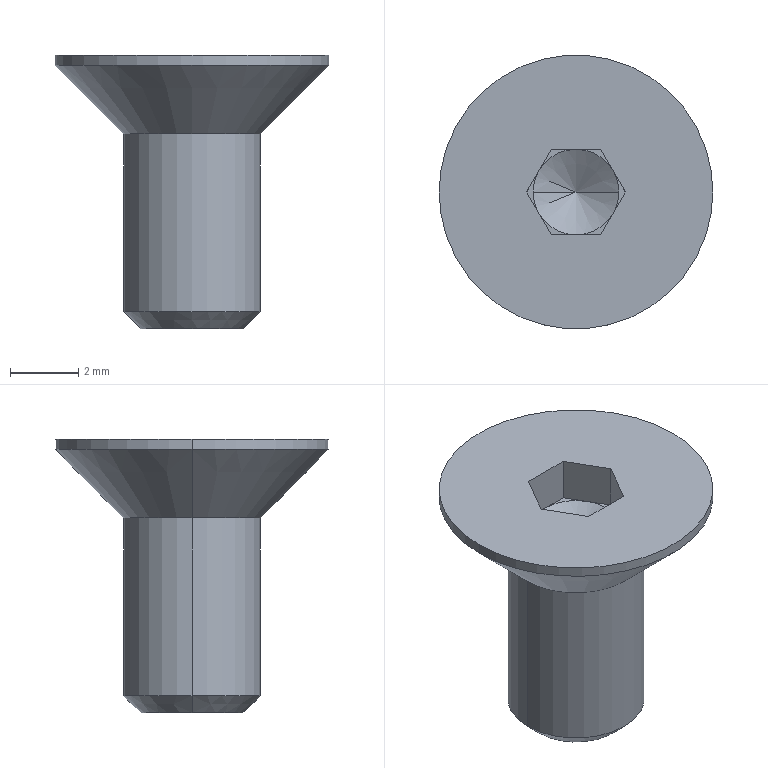Part | NX | features BREP 1 | 1 solid | 24 faces | box 8 x 8 x 8 mm | volume 135.694 mm3 | plane 14 | cone 6 | cylinder 4 | commonest cylinder face diameters 4 x2 8 x2
STEP:
#1=CARTESIAN_POINT('',(0.,0.,-2.022));
#2=VERTEX_POINT('',#1);
#3=CARTESIAN_POINT('',(-1.25,0.,-1.3));
#4=VERTEX_POINT('',#3);
#5=CARTESIAN_POINT('',(-1.25,0.,-1.3));
#6=DIRECTION('',(-0.866,0.,0.5));
#7=VECTOR('',#6,1000.);
#8=LINE('',#5,#7);
#9=EDGE_CURVE('',#2,#4,#8,.T.);
#10=ORIENTED_EDGE('',*,*,#9,.F.);
#11=CARTESIAN_POINT('',(1.25,0.,-1.3));
#12=VERTEX_POINT('',#11);
#13=CARTESIAN_POINT('',(1.25,0.,-1.3));
#14=DIRECTION('',(0.866,0.,0.5));
#15=VECTOR('',#14,1000.);
#16=LINE('',#13,#15);
#17=EDGE_CURVE('',#2,#12,#16,.T.);
#18=ORIENTED_EDGE('',*,*,#17,.T.);
#19=CARTESIAN_POINT('',(1.083,0.625,-1.3));
#20=VERTEX_POINT('',#19);
#21=CARTESIAN_POINT('',(0.,0.,-1.3));
#22=DIRECTION('',(0.,0.,-1.));
#23=DIRECTION('',(-1.,0.,0.));
#24=AXIS2_PLACEMENT_3D('',#21,#22,#23);
#25=CIRCLE('',#24,1.25);
#26=EDGE_CURVE('',#20,#12,#25,.T.);
#27=ORIENTED_EDGE('',*,*,#26,.F.);
#28=CARTESIAN_POINT('',(0.,1.25,-1.3));
#29=VERTEX_POINT('',#28);
#30=CARTESIAN_POINT('',(0.,0.,-1.3));
#31=DIRECTION('',(0.,0.,-1.));
#32=DIRECTION('',(-1.,0.,0.));
#33=AXIS2_PLACEMENT_3D('',#30,#31,#32);
#34=CIRCLE('',#33,1.25);
#35=EDGE_CURVE('',#29,#20,#34,.T.);
#36=ORIENTED_EDGE('',*,*,#35,.F.);
#37=CARTESIAN_POINT('',(-1.083,0.625,-1.3));
#38=VERTEX_POINT('',#37);
#39=CARTESIAN_POINT('',(0.,0.,-1.3));
#40=DIRECTION('',(0.,0.,-1.));
#41=DIRECTION('',(-1.,0.,0.));
#42=AXIS2_PLACEMENT_3D('',#39,#40,#41);
#43=CIRCLE('',#42,1.25);
#44=EDGE_CURVE('',#38,#29,#43,.T.);
#45=ORIENTED_EDGE('',*,*,#44,.F.);
#46=CARTESIAN_POINT('',(0.,0.,-1.3));
#47=DIRECTION('',(0.,0.,-1.));
#48=DIRECTION('',(-1.,0.,0.));
#49=AXIS2_PLACEMENT_3D('',#46,#47,#48);
#50=CIRCLE('',#49,1.25);
#51=EDGE_CURVE('',#4,#38,#50,.T.);
#52=ORIENTED_EDGE('',*,*,#51,.F.);
#53=EDGE_LOOP('',(#10,#18,#27,#36,#45,#52));
#54=FACE_BOUND('',#53,.T.);
#55=CARTESIAN_POINT('',(0.,0.,-1.3));
#56=DIRECTION('',(0.,0.,1.));
#57=DIRECTION('',(-1.,0.,0.));
#58=AXIS2_PLACEMENT_3D('',#55,#56,#57);
#59=CONICAL_SURFACE('',#58,1.25,1.047);
#60=ADVANCED_FACE('',(#54),#59,.F.);
#61=CARTESIAN_POINT('',(-1.5,0.,-8.));
#62=VERTEX_POINT('',#61);
#63=CARTESIAN_POINT('',(1.5,0.,-8.));
#64=VERTEX_POINT('',#63);
#65=CARTESIAN_POINT('',(0.,0.,-8.));
#66=DIRECTION('',(0.,0.,1.));
#67=DIRECTION('',(1.,0.,0.));
#68=AXIS2_PLACEMENT_3D('',#65,#66,#67);
#69=CIRCLE('',#68,1.5);
#70=EDGE_CURVE('',#62,#64,#69,.T.);
#71=ORIENTED_EDGE('',*,*,#70,.T.);
#72=CARTESIAN_POINT('',(2.,0.,-7.5));
#73=VERTEX_POINT('',#72);
#74=CARTESIAN_POINT('',(1.5,0.,-8.));
#75=DIRECTION('',(0.7071,0.,0.7071));
#76=VECTOR('',#75,1000.);
#77=LINE('',#74,#76);
#78=EDGE_CURVE('',#64,#73,#77,.T.);
#79=ORIENTED_EDGE('',*,*,#78,.T.);
#80=CARTESIAN_POINT('',(-2.,0.,-7.5));
#81=VERTEX_POINT('',#80);
#82=CARTESIAN_POINT('',(0.,0.,-7.5));
#83=DIRECTION('',(0.,0.,-1.));
#84=DIRECTION('',(1.,0.,0.));
#85=AXIS2_PLACEMENT_3D('',#82,#83,#84);
#86=CIRCLE('',#85,2.);
#87=EDGE_CURVE('',#73,#81,#86,.T.);
#88=ORIENTED_EDGE('',*,*,#87,.T.);
#89=CARTESIAN_POINT('',(-1.5,0.,-8.));
#90=DIRECTION('',(-0.7071,0.,0.7071));
#91=VECTOR('',#90,1000.);
#92=LINE('',#89,#91);
#93=EDGE_CURVE('',#62,#81,#92,.T.);
#94=ORIENTED_EDGE('',*,*,#93,.F.);
#95=EDGE_LOOP('',(#71,#79,#88,#94));
#96=FACE_BOUND('',#95,.T.);
#97=CARTESIAN_POINT('',(0.,0.,-8.));
#98=DIRECTION('',(0.,0.,1.));
#99=DIRECTION('',(-1.,0.,0.));
#100=AXIS2_PLACEMENT_3D('',#97,#98,#99);
#101=CONICAL_SURFACE('',#100,1.5,0.7854);
#102=ADVANCED_FACE('',(#96),#101,.T.);
#103=ORIENTED_EDGE('',*,*,#87,.F.);
#104=CARTESIAN_POINT('',(2.,0.,-2.3));
#105=VERTEX_POINT('',#104);
#106=CARTESIAN_POINT('',(2.,0.,-8.));
#107=DIRECTION('',(0.,0.,1.));
#108=VECTOR('',#107,1000.);
#109=LINE('',#106,#108);
#110=EDGE_CURVE('',#73,#105,#109,.T.);
#111=ORIENTED_EDGE('',*,*,#110,.T.);
#112=CARTESIAN_POINT('',(-2.,0.,-2.3));
#113=VERTEX_POINT('',#112);
#114=CARTESIAN_POINT('',(0.,0.,-2.3));
#115=DIRECTION('',(0.,0.,1.));
#116=DIRECTION('',(1.,0.,0.));
#117=AXIS2_PLACEMENT_3D('',#114,#115,#116);
#118=CIRCLE('',#117,2.);
#119=EDGE_CURVE('',#113,#105,#118,.T.);
#120=ORIENTED_EDGE('',*,*,#119,.F.);
#121=CARTESIAN_POINT('',(-2.,0.,-8.));
#122=DIRECTION('',(0.,0.,1.));
#123=VECTOR('',#122,1000.);
#124=LINE('',#121,#123);
#125=EDGE_CURVE('',#81,#113,#124,.T.);
#126=ORIENTED_EDGE('',*,*,#125,.F.);
#127=EDGE_LOOP('',(#103,#111,#120,#126));
#128=FACE_BOUND('',#127,.T.);
#129=CARTESIAN_POINT('',(0.,0.,-8.));
#130=DIRECTION('',(0.,0.,1.));
#131=DIRECTION('',(-1.,0.,0.));
#132=AXIS2_PLACEMENT_3D('',#129,#130,#131);
#133=CYLINDRICAL_SURFACE('',#132,2.);
#134=ADVANCED_FACE('',(#128),#133,.T.);
#135=ORIENTED_EDGE('',*,*,#119,.T.);
#136=CARTESIAN_POINT('',(4.,0.,-0.3));
#137=VERTEX_POINT('',#136);
#138=CARTESIAN_POINT('',(2.,0.,-2.3));
#139=DIRECTION('',(0.7071,0.,0.7071));
#140=VECTOR('',#139,1000.);
#141=LINE('',#138,#140);
#142=EDGE_CURVE('',#105,#137,#141,.T.);
#143=ORIENTED_EDGE('',*,*,#142,.T.);
#144=CARTESIAN_POINT('',(-4.,0.,-0.3));
#145=VERTEX_POINT('',#144);
#146=CARTESIAN_POINT('',(0.,0.,-0.3));
#147=DIRECTION('',(0.,0.,-1.));
#148=DIRECTION('',(1.,0.,0.));
#149=AXIS2_PLACEMENT_3D('',#146,#147,#148);
#150=CIRCLE('',#149,4.);
#151=EDGE_CURVE('',#137,#145,#150,.T.);
#152=ORIENTED_EDGE('',*,*,#151,.T.);
#153=CARTESIAN_POINT('',(-2.,0.,-2.3));
#154=DIRECTION('',(-0.7071,0.,0.7071));
#155=VECTOR('',#154,1000.);
#156=LINE('',#153,#155);
#157=EDGE_CURVE('',#113,#145,#156,.T.);
#158=ORIENTED_EDGE('',*,*,#157,.F.);
#159=EDGE_LOOP('',(#135,#143,#152,#158));
#160=FACE_BOUND('',#159,.T.);
#161=CARTESIAN_POINT('',(0.,0.,-2.3));
#162=DIRECTION('',(0.,0.,1.));
#163=DIRECTION('',(-1.,0.,0.));
#164=AXIS2_PLACEMENT_3D('',#161,#162,#163);
#165=CONICAL_SURFACE('',#164,2.,0.7854);
#166=ADVANCED_FACE('',(#160),#165,.T.);
#167=ORIENTED_EDGE('',*,*,#151,.F.);
#168=CARTESIAN_POINT('',(4.,0.,0.));
#169=VERTEX_POINT('',#168);
#170=CARTESIAN_POINT('',(4.,0.,-2.3));
#171=DIRECTION('',(0.,0.,1.));
#172=VECTOR('',#171,1000.);
#173=LINE('',#170,#172);
#174=EDGE_CURVE('',#137,#169,#173,.T.);
#175=ORIENTED_EDGE('',*,*,#174,.T.);
#176=CARTESIAN_POINT('',(-4.,0.,0.));
#177=VERTEX_POINT('',#176);
#178=CARTESIAN_POINT('',(0.,0.,0.));
#179=DIRECTION('',(0.,0.,1.));
#180=DIRECTION('',(1.,0.,0.));
#181=AXIS2_PLACEMENT_3D('',#178,#179,#180);
#182=CIRCLE('',#181,4.);
#183=EDGE_CURVE('',#177,#169,#182,.T.);
#184=ORIENTED_EDGE('',*,*,#183,.F.);
#185=CARTESIAN_POINT('',(-4.,0.,-2.3));
#186=DIRECTION('',(0.,0.,1.));
#187=VECTOR('',#186,1000.);
#188=LINE('',#185,#187);
#189=EDGE_CURVE('',#145,#177,#188,.T.);
#190=ORIENTED_EDGE('',*,*,#189,.F.);
#191=EDGE_LOOP('',(#167,#175,#184,#190));
#192=FACE_BOUND('',#191,.T.);
#193=CARTESIAN_POINT('',(0.,0.,-2.3));
#194=DIRECTION('',(0.,0.,1.));
#195=DIRECTION('',(-1.,0.,0.));
#196=AXIS2_PLACEMENT_3D('',#193,#194,#195);
#197=CYLINDRICAL_SURFACE('',#196,4.);
#198=ADVANCED_FACE('',(#192),#197,.T.);
#199=ORIENTED_EDGE('',*,*,#44,.T.);
#200=CARTESIAN_POINT('',(-0.7217,1.25,-1.3));
#201=VERTEX_POINT('',#200);
#202=CARTESIAN_POINT('',(-0.7217,1.25,-1.3));
#203=DIRECTION('',(1.,0.,0.));
#204=VECTOR('',#203,1000.);
#205=LINE('',#202,#204);
#206=EDGE_CURVE('',#201,#29,#205,.T.);
#207=ORIENTED_EDGE('',*,*,#206,.F.);
#208=CARTESIAN_POINT('',(-1.443,0.,-1.3));
#209=DIRECTION('',(0.5,0.866,0.));
#210=VECTOR('',#209,1000.);
#211=LINE('',#208,#210);
#212=EDGE_CURVE('',#38,#201,#211,.T.);
#213=ORIENTED_EDGE('',*,*,#212,.F.);
#214=EDGE_LOOP('',(#199,#207,#213));
#215=FACE_BOUND('',#214,.T.);
#216=CARTESIAN_POINT('',(0.,0.,-1.3));
#217=DIRECTION('',(0.,0.,1.));
#218=DIRECTION('',(1.,0.,0.));
#219=AXIS2_PLACEMENT_3D('',#216,#217,#218);
#220=PLANE('',#219);
#221=ADVANCED_FACE('',(#215),#220,.T.);
#222=ORIENTED_EDGE('',*,*,#35,.T.);
#223=CARTESIAN_POINT('',(0.7217,1.25,-1.3));
#224=VERTEX_POINT('',#223);
#225=CARTESIAN_POINT('',(0.7217,1.25,-1.3));
#226=DIRECTION('',(0.5,-0.866,0.));
#227=VECTOR('',#226,1000.);
#228=LINE('',#225,#227);
#229=EDGE_CURVE('',#224,#20,#228,.T.);
#230=ORIENTED_EDGE('',*,*,#229,.F.);
#231=CARTESIAN_POINT('',(-0.7217,1.25,-1.3));
#232=DIRECTION('',(1.,0.,0.));
#233=VECTOR('',#232,1000.);
#234=LINE('',#231,#233);
#235=EDGE_CURVE('',#29,#224,#234,.T.);
#236=ORIENTED_EDGE('',*,*,#235,.F.);
#237=EDGE_LOOP('',(#222,#230,#236));
#238=FACE_BOUND('',#237,.T.);
#239=CARTESIAN_POINT('',(0.,0.,-1.3));
#240=DIRECTION('',(0.,0.,1.));
#241=DIRECTION('',(1.,0.,0.));
#242=AXIS2_PLACEMENT_3D('',#239,#240,#241);
#243=PLANE('',#242);
#244=ADVANCED_FACE('',(#238),#243,.T.);
#245=ORIENTED_EDGE('',*,*,#26,.T.);
#246=CARTESIAN_POINT('',(1.083,-0.625,-1.3));
#247=VERTEX_POINT('',#246);
#248=CARTESIAN_POINT('',(0.,0.,-1.3));
#249=DIRECTION('',(0.,0.,-1.));
#250=DIRECTION('',(-1.,0.,0.));
#251=AXIS2_PLACEMENT_3D('',#248,#249,#250);
#252=CIRCLE('',#251,1.25);
#253=EDGE_CURVE('',#12,#247,#252,.T.);
#254=ORIENTED_EDGE('',*,*,#253,.T.);
#255=CARTESIAN_POINT('',(1.443,0.,-1.3));
#256=VERTEX_POINT('',#255);
#257=CARTESIAN_POINT('',(1.443,0.,-1.3));
#258=DIRECTION('',(-0.5,-0.866,0.));
#259=VECTOR('',#258,1000.);
#260=LINE('',#257,#259);
#261=EDGE_CURVE('',#256,#247,#260,.T.);
#262=ORIENTED_EDGE('',*,*,#261,.F.);
#263=CARTESIAN_POINT('',(0.7217,1.25,-1.3));
#264=DIRECTION('',(0.5,-0.866,0.));
#265=VECTOR('',#264,1000.);
#266=LINE('',#263,#265);
#267=EDGE_CURVE('',#20,#256,#266,.T.);
#268=ORIENTED_EDGE('',*,*,#267,.F.);
#269=EDGE_LOOP('',(#245,#254,#262,#268));
#270=FACE_BOUND('',#269,.T.);
#271=CARTESIAN_POINT('',(0.,0.,-1.3));
#272=DIRECTION('',(0.,0.,1.));
#273=DIRECTION('',(1.,0.,0.));
#274=AXIS2_PLACEMENT_3D('',#271,#272,#273);
#275=PLANE('',#274);
#276=ADVANCED_FACE('',(#270),#275,.T.);
#277=CARTESIAN_POINT('',(0.,-1.25,-1.3));
#278=VERTEX_POINT('',#277);
#279=CARTESIAN_POINT('',(0.,0.,-1.3));
#280=DIRECTION('',(0.,0.,-1.));
#281=DIRECTION('',(-1.,0.,0.));
#282=AXIS2_PLACEMENT_3D('',#279,#280,#281);
#283=CIRCLE('',#282,1.25);
#284=EDGE_CURVE('',#247,#278,#283,.T.);
#285=ORIENTED_EDGE('',*,*,#284,.T.);
#286=CARTESIAN_POINT('',(0.7217,-1.25,-1.3));
#287=VERTEX_POINT('',#286);
#288=CARTESIAN_POINT('',(0.7217,-1.25,-1.3));
#289=DIRECTION('',(-1.,0.,0.));
#290=VECTOR('',#289,1000.);
#291=LINE('',#288,#290);
#292=EDGE_CURVE('',#287,#278,#291,.T.);
#293=ORIENTED_EDGE('',*,*,#292,.F.);
#294=CARTESIAN_POINT('',(1.443,0.,-1.3));
#295=DIRECTION('',(-0.5,-0.866,0.));
#296=VECTOR('',#295,1000.);
#297=LINE('',#294,#296);
#298=EDGE_CURVE('',#247,#287,#297,.T.);
#299=ORIENTED_EDGE('',*,*,#298,.F.);
#300=EDGE_LOOP('',(#285,#293,#299));
#301=FACE_BOUND('',#300,.T.);
#302=CARTESIAN_POINT('',(0.,0.,-1.3));
#303=DIRECTION('',(0.,0.,1.));
#304=DIRECTION('',(1.,0.,0.));
#305=AXIS2_PLACEMENT_3D('',#302,#303,#304);
#306=PLANE('',#305);
#307=ADVANCED_FACE('',(#301),#306,.T.);
#308=CARTESIAN_POINT('',(-1.083,-0.625,-1.3));
#309=VERTEX_POINT('',#308);
#310=CARTESIAN_POINT('',(0.,0.,-1.3));
#311=DIRECTION('',(0.,0.,-1.));
#312=DIRECTION('',(-1.,0.,0.));
#313=AXIS2_PLACEMENT_3D('',#310,#311,#312);
#314=CIRCLE('',#313,1.25);
#315=EDGE_CURVE('',#278,#309,#314,.T.);
#316=ORIENTED_EDGE('',*,*,#315,.T.);
#317=CARTESIAN_POINT('',(-0.7217,-1.25,-1.3));
#318=VERTEX_POINT('',#317);
#319=CARTESIAN_POINT('',(-0.7217,-1.25,-1.3));
#320=DIRECTION('',(-0.5,0.866,0.));
#321=VECTOR('',#320,1000.);
#322=LINE('',#319,#321);
#323=EDGE_CURVE('',#318,#309,#322,.T.);
#324=ORIENTED_EDGE('',*,*,#323,.F.);
#325=CARTESIAN_POINT('',(0.7217,-1.25,-1.3));
#326=DIRECTION('',(-1.,0.,0.));
#327=VECTOR('',#326,1000.);
#328=LINE('',#325,#327);
#329=EDGE_CURVE('',#278,#318,#328,.T.);
#330=ORIENTED_EDGE('',*,*,#329,.F.);
#331=EDGE_LOOP('',(#316,#324,#330));
#332=FACE_BOUND('',#331,.T.);
#333=CARTESIAN_POINT('',(0.,0.,-1.3));
#334=DIRECTION('',(0.,0.,1.));
#335=DIRECTION('',(1.,0.,0.));
#336=AXIS2_PLACEMENT_3D('',#333,#334,#335);
#337=PLANE('',#336);
#338=ADVANCED_FACE('',(#332),#337,.T.);
#339=ORIENTED_EDGE('',*,*,#174,.F.);
#340=CARTESIAN_POINT('',(0.,0.,-0.3));
#341=DIRECTION('',(0.,0.,-1.));
#342=DIRECTION('',(1.,0.,0.));
#343=AXIS2_PLACEMENT_3D('',#340,#341,#342);
#344=CIRCLE('',#343,4.);
#345=EDGE_CURVE('',#145,#137,#344,.T.);
#346=ORIENTED_EDGE('',*,*,#345,.F.);
#347=ORIENTED_EDGE('',*,*,#189,.T.);
#348=CARTESIAN_POINT('',(0.,0.,0.));
#349=DIRECTION('',(0.,0.,1.));
#350=DIRECTION('',(1.,0.,0.));
#351=AXIS2_PLACEMENT_3D('',#348,#349,#350);
#352=CIRCLE('',#351,4.);
#353=EDGE_CURVE('',#169,#177,#352,.T.);
#354=ORIENTED_EDGE('',*,*,#353,.F.);
#355=EDGE_LOOP('',(#339,#346,#347,#354));
#356=FACE_BOUND('',#355,.T.);
#357=CARTESIAN_POINT('',(0.,0.,-2.3));
#358=DIRECTION('',(0.,0.,1.));
#359=DIRECTION('',(-1.,0.,0.));
#360=AXIS2_PLACEMENT_3D('',#357,#358,#359);
#361=CYLINDRICAL_SURFACE('',#360,4.);
#362=ADVANCED_FACE('',(#356),#361,.T.);
#363=ORIENTED_EDGE('',*,*,#183,.T.);
#364=ORIENTED_EDGE('',*,*,#353,.T.);
#365=EDGE_LOOP('',(#363,#364));
#366=FACE_BOUND('',#365,.T.);
#367=CARTESIAN_POINT('',(-0.7217,1.25,0.));
#368=VERTEX_POINT('',#367);
#369=CARTESIAN_POINT('',(0.7217,1.25,0.));
#370=VERTEX_POINT('',#369);
#371=CARTESIAN_POINT('',(-0.7217,1.25,0.));
#372=DIRECTION('',(1.,0.,0.));
#373=VECTOR('',#372,1000.);
#374=LINE('',#371,#373);
#375=EDGE_CURVE('',#368,#370,#374,.T.);
#376=ORIENTED_EDGE('',*,*,#375,.T.);
#377=CARTESIAN_POINT('',(1.443,0.,0.));
#378=VERTEX_POINT('',#377);
#379=CARTESIAN_POINT('',(0.7217,1.25,0.));
#380=DIRECTION('',(0.5,-0.866,0.));
#381=VECTOR('',#380,1000.);
#382=LINE('',#379,#381);
#383=EDGE_CURVE('',#370,#378,#382,.T.);
#384=ORIENTED_EDGE('',*,*,#383,.T.);
#385=CARTESIAN_POINT('',(0.7217,-1.25,0.));
#386=VERTEX_POINT('',#385);
#387=CARTESIAN_POINT('',(1.443,0.,0.));
#388=DIRECTION('',(-0.5,-0.866,0.));
#389=VECTOR('',#388,1000.);
#390=LINE('',#387,#389);
#391=EDGE_CURVE('',#378,#386,#390,.T.);
#392=ORIENTED_EDGE('',*,*,#391,.T.);
#393=CARTESIAN_POINT('',(-0.7217,-1.25,0.));
#394=VERTEX_POINT('',#393);
#395=CARTESIAN_POINT('',(0.7217,-1.25,0.));
#396=DIRECTION('',(-1.,0.,0.));
#397=VECTOR('',#396,1000.);
#398=LINE('',#395,#397);
#399=EDGE_CURVE('',#386,#394,#398,.T.);
#400=ORIENTED_EDGE('',*,*,#399,.T.);
#401=CARTESIAN_POINT('',(-1.443,0.,0.));
#402=VERTEX_POINT('',#401);
#403=CARTESIAN_POINT('',(-0.7217,-1.25,0.));
#404=DIRECTION('',(-0.5,0.866,0.));
#405=VECTOR('',#404,1000.);
#406=LINE('',#403,#405);
#407=EDGE_CURVE('',#394,#402,#406,.T.);
#408=ORIENTED_EDGE('',*,*,#407,.T.);
#409=CARTESIAN_POINT('',(-1.443,0.,0.));
#410=DIRECTION('',(0.5,0.866,0.));
#411=VECTOR('',#410,1000.);
#412=LINE('',#409,#411);
#413=EDGE_CURVE('',#402,#368,#412,.T.);
#414=ORIENTED_EDGE('',*,*,#413,.T.);
#415=EDGE_LOOP('',(#376,#384,#392,#400,#408,#414));
#416=FACE_BOUND('',#415,.T.);
#417=CARTESIAN_POINT('',(0.,0.,0.));
#418=DIRECTION('',(0.,0.,-1.));
#419=DIRECTION('',(0.,-1.,0.));
#420=AXIS2_PLACEMENT_3D('',#417,#418,#419);
#421=PLANE('',#420);
#422=ADVANCED_FACE('',(#366,#416),#421,.F.);
#423=ORIENTED_EDGE('',*,*,#142,.F.);
#424=CARTESIAN_POINT('',(0.,0.,-2.3));
#425=DIRECTION('',(0.,0.,1.));
#426=DIRECTION('',(1.,0.,0.));
#427=AXIS2_PLACEMENT_3D('',#424,#425,#426);
#428=CIRCLE('',#427,2.);
#429=EDGE_CURVE('',#105,#113,#428,.T.);
#430=ORIENTED_EDGE('',*,*,#429,.T.);
#431=ORIENTED_EDGE('',*,*,#157,.T.);
#432=ORIENTED_EDGE('',*,*,#345,.T.);
#433=EDGE_LOOP('',(#423,#430,#431,#432));
#434=FACE_BOUND('',#433,.T.);
#435=CARTESIAN_POINT('',(0.,0.,-2.3));
#436=DIRECTION('',(0.,0.,1.));
#437=DIRECTION('',(-1.,0.,0.));
#438=AXIS2_PLACEMENT_3D('',#435,#436,#437);
#439=CONICAL_SURFACE('',#438,2.,0.7854);
#440=ADVANCED_FACE('',(#434),#439,.T.);
#441=ORIENTED_EDGE('',*,*,#110,.F.);
#442=CARTESIAN_POINT('',(0.,0.,-7.5));
#443=DIRECTION('',(0.,0.,-1.));
#444=DIRECTION('',(1.,0.,0.));
#445=AXIS2_PLACEMENT_3D('',#442,#443,#444);
#446=CIRCLE('',#445,2.);
#447=EDGE_CURVE('',#81,#73,#446,.T.);
#448=ORIENTED_EDGE('',*,*,#447,.F.);
#449=ORIENTED_EDGE('',*,*,#125,.T.);
#450=ORIENTED_EDGE('',*,*,#429,.F.);
#451=EDGE_LOOP('',(#441,#448,#449,#450));
#452=FACE_BOUND('',#451,.T.);
#453=CARTESIAN_POINT('',(0.,0.,-8.));
#454=DIRECTION('',(0.,0.,1.));
#455=DIRECTION('',(-1.,0.,0.));
#456=AXIS2_PLACEMENT_3D('',#453,#454,#455);
#457=CYLINDRICAL_SURFACE('',#456,2.);
#458=ADVANCED_FACE('',(#452),#457,.T.);
#459=ORIENTED_EDGE('',*,*,#70,.F.);
#460=CARTESIAN_POINT('',(0.,0.,-8.));
#461=DIRECTION('',(0.,0.,1.));
#462=DIRECTION('',(1.,0.,0.));
#463=AXIS2_PLACEMENT_3D('',#460,#461,#462);
#464=CIRCLE('',#463,1.5);
#465=EDGE_CURVE('',#64,#62,#464,.T.);
#466=ORIENTED_EDGE('',*,*,#465,.F.);
#467=EDGE_LOOP('',(#459,#466));
#468=FACE_BOUND('',#467,.T.);
#469=CARTESIAN_POINT('',(0.,0.,-8.));
#470=DIRECTION('',(0.,0.,-1.));
#471=DIRECTION('',(0.,-1.,0.));
#472=AXIS2_PLACEMENT_3D('',#469,#470,#471);
#473=PLANE('',#472);
#474=ADVANCED_FACE('',(#468),#473,.T.);
#475=ORIENTED_EDGE('',*,*,#78,.F.);
#476=ORIENTED_EDGE('',*,*,#465,.T.);
#477=ORIENTED_EDGE('',*,*,#93,.T.);
#478=ORIENTED_EDGE('',*,*,#447,.T.);
#479=EDGE_LOOP('',(#475,#476,#477,#478));
#480=FACE_BOUND('',#479,.T.);
#481=CARTESIAN_POINT('',(0.,0.,-8.));
#482=DIRECTION('',(0.,0.,1.));
#483=DIRECTION('',(-1.,0.,0.));
#484=AXIS2_PLACEMENT_3D('',#481,#482,#483);
#485=CONICAL_SURFACE('',#484,1.5,0.7854);
#486=ADVANCED_FACE('',(#480),#485,.T.);
#487=ORIENTED_EDGE('',*,*,#413,.F.);
#488=CARTESIAN_POINT('',(-1.443,0.,-1.3));
#489=VERTEX_POINT('',#488);
#490=CARTESIAN_POINT('',(-1.443,0.,-1.3));
#491=DIRECTION('',(0.,0.,1.));
#492=VECTOR('',#491,1000.);
#493=LINE('',#490,#492);
#494=EDGE_CURVE('',#489,#402,#493,.T.);
#495=ORIENTED_EDGE('',*,*,#494,.F.);
#496=CARTESIAN_POINT('',(-1.443,0.,-1.3));
#497=DIRECTION('',(0.5,0.866,0.));
#498=VECTOR('',#497,1000.);
#499=LINE('',#496,#498);
#500=EDGE_CURVE('',#489,#38,#499,.T.);
#501=ORIENTED_EDGE('',*,*,#500,.T.);
#502=ORIENTED_EDGE('',*,*,#212,.T.);
#503=CARTESIAN_POINT('',(-0.7217,1.25,-1.3));
#504=DIRECTION('',(0.,0.,1.));
#505=VECTOR('',#504,1000.);
#506=LINE('',#503,#505);
#507=EDGE_CURVE('',#201,#368,#506,.T.);
#508=ORIENTED_EDGE('',*,*,#507,.T.);
#509=EDGE_LOOP('',(#487,#495,#501,#502,#508));
#510=FACE_BOUND('',#509,.T.);
#511=CARTESIAN_POINT('',(-1.443,0.,-1.3));
#512=DIRECTION('',(-0.866,0.5,0.));
#513=DIRECTION('',(0.,0.,1.));
#514=AXIS2_PLACEMENT_3D('',#511,#512,#513);
#515=PLANE('',#514);
#516=ADVANCED_FACE('',(#510),#515,.F.);
#517=ORIENTED_EDGE('',*,*,#407,.F.);
#518=CARTESIAN_POINT('',(-0.7217,-1.25,-1.3));
#519=DIRECTION('',(0.,0.,1.));
#520=VECTOR('',#519,1000.);
#521=LINE('',#518,#520);
#522=EDGE_CURVE('',#318,#394,#521,.T.);
#523=ORIENTED_EDGE('',*,*,#522,.F.);
#524=ORIENTED_EDGE('',*,*,#323,.T.);
#525=CARTESIAN_POINT('',(-0.7217,-1.25,-1.3));
#526=DIRECTION('',(-0.5,0.866,0.));
#527=VECTOR('',#526,1000.);
#528=LINE('',#525,#527);
#529=EDGE_CURVE('',#309,#489,#528,.T.);
#530=ORIENTED_EDGE('',*,*,#529,.T.);
#531=ORIENTED_EDGE('',*,*,#494,.T.);
#532=EDGE_LOOP('',(#517,#523,#524,#530,#531));
#533=FACE_BOUND('',#532,.T.);
#534=CARTESIAN_POINT('',(-0.7217,-1.25,-1.3));
#535=DIRECTION('',(-0.866,-0.5,0.));
#536=DIRECTION('',(-0.5,0.866,0.));
#537=AXIS2_PLACEMENT_3D('',#534,#535,#536);
#538=PLANE('',#537);
#539=ADVANCED_FACE('',(#533),#538,.F.);
#540=ORIENTED_EDGE('',*,*,#399,.F.);
#541=CARTESIAN_POINT('',(0.7217,-1.25,-1.3));
#542=DIRECTION('',(0.,0.,1.));
#543=VECTOR('',#542,1000.);
#544=LINE('',#541,#543);
#545=EDGE_CURVE('',#287,#386,#544,.T.);
#546=ORIENTED_EDGE('',*,*,#545,.F.);
#547=ORIENTED_EDGE('',*,*,#292,.T.);
#548=ORIENTED_EDGE('',*,*,#329,.T.);
#549=ORIENTED_EDGE('',*,*,#522,.T.);
#550=EDGE_LOOP('',(#540,#546,#547,#548,#549));
#551=FACE_BOUND('',#550,.T.);
#552=CARTESIAN_POINT('',(0.7217,-1.25,-1.3));
#553=DIRECTION('',(0.,-1.,0.));
#554=DIRECTION('',(0.,0.,-1.));
#555=AXIS2_PLACEMENT_3D('',#552,#553,#554);
#556=PLANE('',#555);
#557=ADVANCED_FACE('',(#551),#556,.F.);
#558=ORIENTED_EDGE('',*,*,#391,.F.);
#559=CARTESIAN_POINT('',(1.443,0.,-1.3));
#560=DIRECTION('',(0.,0.,1.));
#561=VECTOR('',#560,1000.);
#562=LINE('',#559,#561);
#563=EDGE_CURVE('',#256,#378,#562,.T.);
#564=ORIENTED_EDGE('',*,*,#563,.F.);
#565=ORIENTED_EDGE('',*,*,#261,.T.);
#566=ORIENTED_EDGE('',*,*,#298,.T.);
#567=ORIENTED_EDGE('',*,*,#545,.T.);
#568=EDGE_LOOP('',(#558,#564,#565,#566,#567));
#569=FACE_BOUND('',#568,.T.);
#570=CARTESIAN_POINT('',(1.443,0.,-1.3));
#571=DIRECTION('',(0.866,-0.5,0.));
#572=DIRECTION('',(0.,0.,-1.));
#573=AXIS2_PLACEMENT_3D('',#570,#571,#572);
#574=PLANE('',#573);
#575=ADVANCED_FACE('',(#569),#574,.F.);
#576=ORIENTED_EDGE('',*,*,#383,.F.);
#577=CARTESIAN_POINT('',(0.7217,1.25,-1.3));
#578=DIRECTION('',(0.,0.,1.));
#579=VECTOR('',#578,1000.);
#580=LINE('',#577,#579);
#581=EDGE_CURVE('',#224,#370,#580,.T.);
#582=ORIENTED_EDGE('',*,*,#581,.F.);
#583=ORIENTED_EDGE('',*,*,#229,.T.);
#584=ORIENTED_EDGE('',*,*,#267,.T.);
#585=ORIENTED_EDGE('',*,*,#563,.T.);
#586=EDGE_LOOP('',(#576,#582,#583,#584,#585));
#587=FACE_BOUND('',#586,.T.);
#588=CARTESIAN_POINT('',(0.7217,1.25,-1.3));
#589=DIRECTION('',(0.866,0.5,0.));
#590=DIRECTION('',(0.,0.,-1.));
#591=AXIS2_PLACEMENT_3D('',#588,#589,#590);
#592=PLANE('',#591);
#593=ADVANCED_FACE('',(#587),#592,.F.);
#594=ORIENTED_EDGE('',*,*,#375,.F.);
#595=ORIENTED_EDGE('',*,*,#507,.F.);
#596=ORIENTED_EDGE('',*,*,#206,.T.);
#597=ORIENTED_EDGE('',*,*,#235,.T.);
#598=ORIENTED_EDGE('',*,*,#581,.T.);
#599=EDGE_LOOP('',(#594,#595,#596,#597,#598));
#600=FACE_BOUND('',#599,.T.);
#601=CARTESIAN_POINT('',(-0.7217,1.25,-1.3));
#602=DIRECTION('',(0.,1.,0.));
#603=DIRECTION('',(1.,0.,0.));
#604=AXIS2_PLACEMENT_3D('',#601,#602,#603);
#605=PLANE('',#604);
#606=ADVANCED_FACE('',(#600),#605,.F.);
#607=CARTESIAN_POINT('',(0.,0.,-1.3));
#608=DIRECTION('',(0.,0.,-1.));
#609=DIRECTION('',(-1.,0.,0.));
#610=AXIS2_PLACEMENT_3D('',#607,#608,#609);
#611=CIRCLE('',#610,1.25);
#612=EDGE_CURVE('',#309,#4,#611,.T.);
#613=ORIENTED_EDGE('',*,*,#612,.T.);
#614=ORIENTED_EDGE('',*,*,#51,.T.);
#615=ORIENTED_EDGE('',*,*,#500,.F.);
#616=ORIENTED_EDGE('',*,*,#529,.F.);
#617=EDGE_LOOP('',(#613,#614,#615,#616));
#618=FACE_BOUND('',#617,.T.);
#619=CARTESIAN_POINT('',(0.,0.,-1.3));
#620=DIRECTION('',(0.,0.,1.));
#621=DIRECTION('',(1.,0.,0.));
#622=AXIS2_PLACEMENT_3D('',#619,#620,#621);
#623=PLANE('',#622);
#624=ADVANCED_FACE('',(#618),#623,.T.);
#625=ORIENTED_EDGE('',*,*,#17,.F.);
#626=ORIENTED_EDGE('',*,*,#9,.T.);
#627=ORIENTED_EDGE('',*,*,#612,.F.);
#628=ORIENTED_EDGE('',*,*,#315,.F.);
#629=ORIENTED_EDGE('',*,*,#284,.F.);
#630=ORIENTED_EDGE('',*,*,#253,.F.);
#631=EDGE_LOOP('',(#625,#626,#627,#628,#629,#630));
#632=FACE_BOUND('',#631,.T.);
#633=CARTESIAN_POINT('',(0.,0.,-1.3));
#634=DIRECTION('',(0.,0.,1.));
#635=DIRECTION('',(-1.,0.,0.));
#636=AXIS2_PLACEMENT_3D('',#633,#634,#635);
#637=CONICAL_SURFACE('',#636,1.25,1.047);
#638=ADVANCED_FACE('',(#632),#637,.F.);
#639=CLOSED_SHELL('',(#60,#102,#134,#166,#198,#221,#244,#276,#307,#338,#362,#422,#440,#458,#474,#486,#516,#539,#557,#575,#593,#606,#624,#638));
#640=MANIFOLD_SOLID_BREP('',#639);
#641=(LENGTH_UNIT()NAMED_UNIT(*)SI_UNIT(.MILLI.,.METRE.));
#642=UNCERTAINTY_MEASURE_WITH_UNIT(LENGTH_MEASURE(0.00001),#641,'','');
#643=(NAMED_UNIT(*)PLANE_ANGLE_UNIT()SI_UNIT($,.RADIAN.));
#644=(NAMED_UNIT(*)SI_UNIT($,.STERADIAN.)SOLID_ANGLE_UNIT());
#645=(GEOMETRIC_REPRESENTATION_CONTEXT(3)GLOBAL_UNCERTAINTY_ASSIGNED_CONTEXT((#642))GLOBAL_UNIT_ASSIGNED_CONTEXT((#641,#643,#644))REPRESENTATION_CONTEXT('',''));
#646=ADVANCED_BREP_SHAPE_REPRESENTATION('',(#640),#645);